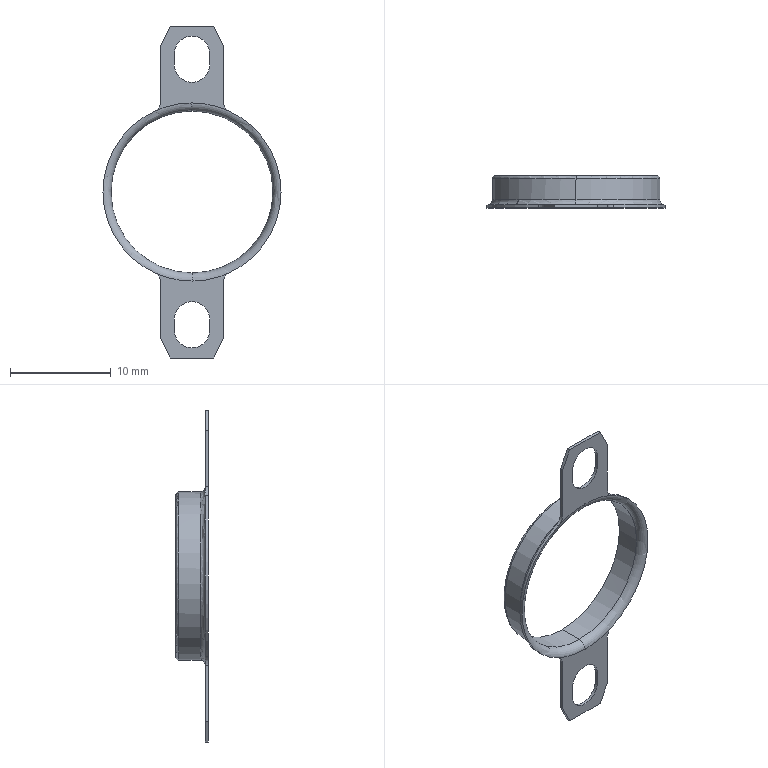Part | STEP file | WENKONGZHIJIA_3_1 | 1 solid | 38 faces | box 17.7 x 3.2 x 33 mm | volume 72.757 mm3 | plane 18 | cylinder 14 | torus 6 | commonest cylinder face diameters 2 x4 3.5 x4 16.1 x2 16.7 x2 17.7 x2
STEP:
#1=CARTESIAN_POINT('',(0.,0.,0.));
#2=DIRECTION('',(0.,0.,1.));
#3=DIRECTION('',(1.,0.,0.));
#4=AXIS2_PLACEMENT_3D('',#1,#2,#3);
#5=CARTESIAN_POINT('',(3.729,0.,8.026));
#6=VERTEX_POINT('',#5);
#7=CARTESIAN_POINT('',(0.,0.,8.85));
#8=VERTEX_POINT('',#7);
#9=CARTESIAN_POINT('',(0.,0.,0.));
#10=DIRECTION('',(0.,-1.,0.));
#11=DIRECTION('',(0.4213,0.,0.9069));
#12=AXIS2_PLACEMENT_3D('',#9,#10,#11);
#13=CIRCLE('',#12,8.85);
#14=EDGE_CURVE('',#6,#8,#13,.T.);
#15=ORIENTED_EDGE('',*,*,#14,.T.);
#16=CARTESIAN_POINT('',(-0.09026,0.,8.85));
#17=VERTEX_POINT('',#16);
#18=CARTESIAN_POINT('',(0.,0.,0.));
#19=DIRECTION('',(0.,1.,0.));
#20=DIRECTION('',(-0.0102,0.,0.9999));
#21=AXIS2_PLACEMENT_3D('',#18,#19,#20);
#22=CIRCLE('',#21,8.85);
#23=EDGE_CURVE('',#17,#8,#22,.T.);
#24=ORIENTED_EDGE('',*,*,#23,.F.);
#25=CARTESIAN_POINT('',(-3.729,0.,8.026));
#26=VERTEX_POINT('',#25);
#27=CARTESIAN_POINT('',(0.,0.,0.));
#28=DIRECTION('',(0.,-1.,0.));
#29=DIRECTION('',(-0.0102,0.,0.9999));
#30=AXIS2_PLACEMENT_3D('',#27,#28,#29);
#31=CIRCLE('',#30,8.85);
#32=EDGE_CURVE('',#17,#26,#31,.T.);
#33=ORIENTED_EDGE('',*,*,#32,.T.);
#34=CARTESIAN_POINT('',(-3.15,0.,8.933));
#35=VERTEX_POINT('',#34);
#36=CARTESIAN_POINT('',(-4.15,0.,8.933));
#37=DIRECTION('',(0.,-1.,0.));
#38=DIRECTION('',(0.4213,0.,-0.9069));
#39=AXIS2_PLACEMENT_3D('',#36,#37,#38);
#40=CIRCLE('',#39,1.);
#41=EDGE_CURVE('',#26,#35,#40,.T.);
#42=ORIENTED_EDGE('',*,*,#41,.T.);
#43=CARTESIAN_POINT('',(-3.15,0.,14.5));
#44=VERTEX_POINT('',#43);
#45=CARTESIAN_POINT('',(-3.15,0.,14.5));
#46=DIRECTION('',(0.,0.,-1.));
#47=VECTOR('',#46,5.567);
#48=LINE('',#45,#47);
#49=EDGE_CURVE('',#44,#35,#48,.T.);
#50=ORIENTED_EDGE('',*,*,#49,.F.);
#51=CARTESIAN_POINT('',(-2.15,0.,16.5));
#52=VERTEX_POINT('',#51);
#53=CARTESIAN_POINT('',(-3.15,0.,14.5));
#54=DIRECTION('',(0.4472,0.,0.8944));
#55=VECTOR('',#54,2.236);
#56=LINE('',#53,#55);
#57=EDGE_CURVE('',#44,#52,#56,.T.);
#58=ORIENTED_EDGE('',*,*,#57,.T.);
#59=CARTESIAN_POINT('',(2.15,0.,16.5));
#60=VERTEX_POINT('',#59);
#61=CARTESIAN_POINT('',(2.15,0.,16.5));
#62=DIRECTION('',(-1.,0.,0.));
#63=VECTOR('',#62,4.3);
#64=LINE('',#61,#63);
#65=EDGE_CURVE('',#60,#52,#64,.T.);
#66=ORIENTED_EDGE('',*,*,#65,.F.);
#67=CARTESIAN_POINT('',(3.15,0.,14.5));
#68=VERTEX_POINT('',#67);
#69=CARTESIAN_POINT('',(2.15,0.,16.5));
#70=DIRECTION('',(0.4472,0.,-0.8944));
#71=VECTOR('',#70,2.236);
#72=LINE('',#69,#71);
#73=EDGE_CURVE('',#60,#68,#72,.T.);
#74=ORIENTED_EDGE('',*,*,#73,.T.);
#75=CARTESIAN_POINT('',(3.15,0.,8.933));
#76=VERTEX_POINT('',#75);
#77=CARTESIAN_POINT('',(3.15,0.,8.933));
#78=DIRECTION('',(0.,0.,1.));
#79=VECTOR('',#78,5.567);
#80=LINE('',#77,#79);
#81=EDGE_CURVE('',#76,#68,#80,.T.);
#82=ORIENTED_EDGE('',*,*,#81,.F.);
#83=CARTESIAN_POINT('',(4.15,0.,8.933));
#84=DIRECTION('',(0.,-1.,0.));
#85=DIRECTION('',(-1.,0.,0.));
#86=AXIS2_PLACEMENT_3D('',#83,#84,#85);
#87=CIRCLE('',#86,1.);
#88=EDGE_CURVE('',#76,#6,#87,.T.);
#89=ORIENTED_EDGE('',*,*,#88,.T.);
#90=EDGE_LOOP('',(#15,#24,#33,#42,#50,#58,#66,#74,#82,#89));
#91=FACE_OUTER_BOUND('',#90,.F.);
#92=CARTESIAN_POINT('',(1.75,0.,13.75));
#93=VERTEX_POINT('',#92);
#94=CARTESIAN_POINT('',(0.,0.,15.5));
#95=VERTEX_POINT('',#94);
#96=CARTESIAN_POINT('',(0.,0.,13.75));
#97=DIRECTION('',(0.,-1.,0.));
#98=DIRECTION('',(1.,0.,0.));
#99=AXIS2_PLACEMENT_3D('',#96,#97,#98);
#100=CIRCLE('',#99,1.75);
#101=EDGE_CURVE('',#93,#95,#100,.T.);
#102=ORIENTED_EDGE('',*,*,#101,.T.);
#103=CARTESIAN_POINT('',(-1.75,0.,13.75));
#104=VERTEX_POINT('',#103);
#105=CARTESIAN_POINT('',(0.,0.,13.75));
#106=DIRECTION('',(0.,-1.,0.));
#107=DIRECTION('',(0.,0.,1.));
#108=AXIS2_PLACEMENT_3D('',#105,#106,#107);
#109=CIRCLE('',#108,1.75);
#110=EDGE_CURVE('',#95,#104,#109,.T.);
#111=ORIENTED_EDGE('',*,*,#110,.T.);
#112=CARTESIAN_POINT('',(-1.75,0.,12.65));
#113=VERTEX_POINT('',#112);
#114=CARTESIAN_POINT('',(-1.75,0.,12.65));
#115=DIRECTION('',(0.,0.,1.));
#116=VECTOR('',#115,1.1);
#117=LINE('',#114,#116);
#118=EDGE_CURVE('',#113,#104,#117,.T.);
#119=ORIENTED_EDGE('',*,*,#118,.F.);
#120=CARTESIAN_POINT('',(0.,0.,10.9));
#121=VERTEX_POINT('',#120);
#122=CARTESIAN_POINT('',(0.,0.,12.65));
#123=DIRECTION('',(0.,-1.,0.));
#124=DIRECTION('',(-1.,0.,0.));
#125=AXIS2_PLACEMENT_3D('',#122,#123,#124);
#126=CIRCLE('',#125,1.75);
#127=EDGE_CURVE('',#113,#121,#126,.T.);
#128=ORIENTED_EDGE('',*,*,#127,.T.);
#129=CARTESIAN_POINT('',(1.75,0.,12.65));
#130=VERTEX_POINT('',#129);
#131=CARTESIAN_POINT('',(0.,0.,12.65));
#132=DIRECTION('',(0.,-1.,0.));
#133=DIRECTION('',(0.,0.,-1.));
#134=AXIS2_PLACEMENT_3D('',#131,#132,#133);
#135=CIRCLE('',#134,1.75);
#136=EDGE_CURVE('',#121,#130,#135,.T.);
#137=ORIENTED_EDGE('',*,*,#136,.T.);
#138=CARTESIAN_POINT('',(1.75,0.,13.75));
#139=DIRECTION('',(0.,0.,-1.));
#140=VECTOR('',#139,1.1);
#141=LINE('',#138,#140);
#142=EDGE_CURVE('',#93,#130,#141,.T.);
#143=ORIENTED_EDGE('',*,*,#142,.F.);
#144=EDGE_LOOP('',(#102,#111,#119,#128,#137,#143));
#145=FACE_BOUND('',#144,.F.);
#146=CARTESIAN_POINT('',(0.,0.,0.));
#147=DIRECTION('',(0.,1.,0.));
#148=DIRECTION('',(1.,0.,0.));
#149=AXIS2_PLACEMENT_3D('',#146,#147,#148);
#150=PLANE('',#149);
#151=ADVANCED_FACE('',(#91,#145),#150,.F.);
#152=ORIENTED_EDGE('',*,*,#14,.F.);
#153=CARTESIAN_POINT('',(8.85,0.,0.));
#154=VERTEX_POINT('',#153);
#155=CARTESIAN_POINT('',(0.,0.,0.));
#156=DIRECTION('',(0.,1.,0.));
#157=DIRECTION('',(0.4213,0.,0.9069));
#158=AXIS2_PLACEMENT_3D('',#155,#156,#157);
#159=CIRCLE('',#158,8.85);
#160=EDGE_CURVE('',#6,#154,#159,.T.);
#161=ORIENTED_EDGE('',*,*,#160,.T.);
#162=CARTESIAN_POINT('',(3.729,0.,-8.026));
#163=VERTEX_POINT('',#162);
#164=CARTESIAN_POINT('',(0.,0.,0.));
#165=DIRECTION('',(0.,1.,0.));
#166=DIRECTION('',(1.,0.,0.));
#167=AXIS2_PLACEMENT_3D('',#164,#165,#166);
#168=CIRCLE('',#167,8.85);
#169=EDGE_CURVE('',#154,#163,#168,.T.);
#170=ORIENTED_EDGE('',*,*,#169,.T.);
#171=CARTESIAN_POINT('',(0.09026,0.,-8.85));
#172=VERTEX_POINT('',#171);
#173=CARTESIAN_POINT('',(0.,0.,0.));
#174=DIRECTION('',(0.,-1.,0.));
#175=DIRECTION('',(0.0102,0.,-0.9999));
#176=AXIS2_PLACEMENT_3D('',#173,#174,#175);
#177=CIRCLE('',#176,8.85);
#178=EDGE_CURVE('',#172,#163,#177,.T.);
#179=ORIENTED_EDGE('',*,*,#178,.F.);
#180=CARTESIAN_POINT('',(0.,0.,-8.85));
#181=VERTEX_POINT('',#180);
#182=CARTESIAN_POINT('',(0.,0.,0.));
#183=DIRECTION('',(0.,1.,0.));
#184=DIRECTION('',(0.0102,0.,-0.9999));
#185=AXIS2_PLACEMENT_3D('',#182,#183,#184);
#186=CIRCLE('',#185,8.85);
#187=EDGE_CURVE('',#172,#181,#186,.T.);
#188=ORIENTED_EDGE('',*,*,#187,.T.);
#189=CARTESIAN_POINT('',(0.,0.8,-8.05));
#190=VERTEX_POINT('',#189);
#191=CARTESIAN_POINT('',(0.,0.8,-8.85));
#192=DIRECTION('',(-1.,0.,0.));
#193=DIRECTION('',(0.,-1.,0.));
#194=AXIS2_PLACEMENT_3D('',#191,#192,#193);
#195=CIRCLE('',#194,0.8);
#196=EDGE_CURVE('',#181,#190,#195,.T.);
#197=ORIENTED_EDGE('',*,*,#196,.T.);
#198=CARTESIAN_POINT('',(0.08211,0.8,-8.05));
#199=VERTEX_POINT('',#198);
#200=CARTESIAN_POINT('',(0.,0.8,0.));
#201=DIRECTION('',(0.,-1.,0.));
#202=DIRECTION('',(0.,0.,-1.));
#203=AXIS2_PLACEMENT_3D('',#200,#201,#202);
#204=CIRCLE('',#203,8.05);
#205=EDGE_CURVE('',#190,#199,#204,.T.);
#206=ORIENTED_EDGE('',*,*,#205,.T.);
#207=CARTESIAN_POINT('',(0.,0.8,8.05));
#208=VERTEX_POINT('',#207);
#209=CARTESIAN_POINT('',(0.,0.8,0.));
#210=DIRECTION('',(0.,-1.,0.));
#211=DIRECTION('',(0.0102,0.,-0.9999));
#212=AXIS2_PLACEMENT_3D('',#209,#210,#211);
#213=CIRCLE('',#212,8.05);
#214=EDGE_CURVE('',#199,#208,#213,.T.);
#215=ORIENTED_EDGE('',*,*,#214,.T.);
#216=CARTESIAN_POINT('',(0.,0.8,8.85));
#217=DIRECTION('',(1.,0.,0.));
#218=DIRECTION('',(0.,-1.,0.));
#219=AXIS2_PLACEMENT_3D('',#216,#217,#218);
#220=CIRCLE('',#219,0.8);
#221=EDGE_CURVE('',#8,#208,#220,.T.);
#222=ORIENTED_EDGE('',*,*,#221,.F.);
#223=EDGE_LOOP('',(#152,#161,#170,#179,#188,#197,#206,#215,#222));
#224=FACE_OUTER_BOUND('',#223,.F.);
#225=CARTESIAN_POINT('',(0.,0.8,0.));
#226=DIRECTION('',(0.,-1.,0.));
#227=DIRECTION('',(-0.0102,0.,0.9999));
#228=AXIS2_PLACEMENT_3D('',#225,#226,#227);
#229=TOROIDAL_SURFACE('',#228,8.85,0.8);
#230=ADVANCED_FACE('',(#224),#229,.T.);
#231=CARTESIAN_POINT('',(8.85,0.3,0.));
#232=VERTEX_POINT('',#231);
#233=CARTESIAN_POINT('',(3.729,0.3,8.026));
#234=VERTEX_POINT('',#233);
#235=CARTESIAN_POINT('',(0.,0.3,0.));
#236=DIRECTION('',(0.,-1.,0.));
#237=DIRECTION('',(1.,0.,0.));
#238=AXIS2_PLACEMENT_3D('',#235,#236,#237);
#239=CIRCLE('',#238,8.85);
#240=EDGE_CURVE('',#232,#234,#239,.T.);
#241=ORIENTED_EDGE('',*,*,#240,.F.);
#242=CARTESIAN_POINT('',(3.729,0.3,-8.026));
#243=VERTEX_POINT('',#242);
#244=CARTESIAN_POINT('',(0.,0.3,0.));
#245=DIRECTION('',(0.,-1.,0.));
#246=DIRECTION('',(0.4213,0.,-0.9069));
#247=AXIS2_PLACEMENT_3D('',#244,#245,#246);
#248=CIRCLE('',#247,8.85);
#249=EDGE_CURVE('',#243,#232,#248,.T.);
#250=ORIENTED_EDGE('',*,*,#249,.F.);
#251=CARTESIAN_POINT('',(3.729,0.3,-8.026));
#252=DIRECTION('',(0.,-1.,0.));
#253=VECTOR('',#252,0.3);
#254=LINE('',#251,#253);
#255=EDGE_CURVE('',#243,#163,#254,.T.);
#256=ORIENTED_EDGE('',*,*,#255,.T.);
#257=ORIENTED_EDGE('',*,*,#169,.F.);
#258=ORIENTED_EDGE('',*,*,#160,.F.);
#259=CARTESIAN_POINT('',(3.729,0.,8.026));
#260=DIRECTION('',(0.,1.,0.));
#261=VECTOR('',#260,0.3);
#262=LINE('',#259,#261);
#263=EDGE_CURVE('',#6,#234,#262,.T.);
#264=ORIENTED_EDGE('',*,*,#263,.T.);
#265=EDGE_LOOP('',(#241,#250,#256,#257,#258,#264));
#266=FACE_OUTER_BOUND('',#265,.F.);
#267=CARTESIAN_POINT('',(0.,0.,0.));
#268=DIRECTION('',(0.,1.,0.));
#269=DIRECTION('',(1.,0.,0.));
#270=AXIS2_PLACEMENT_3D('',#267,#268,#269);
#271=CYLINDRICAL_SURFACE('',#270,8.85);
#272=ADVANCED_FACE('',(#266),#271,.T.);
#273=CARTESIAN_POINT('',(0.,0.3,-8.85));
#274=VERTEX_POINT('',#273);
#275=CARTESIAN_POINT('',(0.06126,0.3,-8.85));
#276=VERTEX_POINT('',#275);
#277=CARTESIAN_POINT('',(0.,0.3,0.));
#278=DIRECTION('',(0.,-1.,0.));
#279=DIRECTION('',(0.,0.,-1.));
#280=AXIS2_PLACEMENT_3D('',#277,#278,#279);
#281=CIRCLE('',#280,8.85);
#282=EDGE_CURVE('',#274,#276,#281,.T.);
#283=ORIENTED_EDGE('',*,*,#282,.T.);
#284=CARTESIAN_POINT('',(0.,0.3,0.));
#285=DIRECTION('',(0.,1.,0.));
#286=DIRECTION('',(0.4213,0.,-0.9069));
#287=AXIS2_PLACEMENT_3D('',#284,#285,#286);
#288=CIRCLE('',#287,8.85);
#289=EDGE_CURVE('',#243,#276,#288,.T.);
#290=ORIENTED_EDGE('',*,*,#289,.F.);
#291=ORIENTED_EDGE('',*,*,#249,.T.);
#292=ORIENTED_EDGE('',*,*,#240,.T.);
#293=CARTESIAN_POINT('',(0.,0.3,8.85));
#294=VERTEX_POINT('',#293);
#295=CARTESIAN_POINT('',(0.,0.3,0.));
#296=DIRECTION('',(0.,1.,0.));
#297=DIRECTION('',(0.,0.,1.));
#298=AXIS2_PLACEMENT_3D('',#295,#296,#297);
#299=CIRCLE('',#298,8.85);
#300=EDGE_CURVE('',#294,#234,#299,.T.);
#301=ORIENTED_EDGE('',*,*,#300,.F.);
#302=CARTESIAN_POINT('',(0.,0.8,8.35));
#303=VERTEX_POINT('',#302);
#304=CARTESIAN_POINT('',(0.,0.8,8.85));
#305=DIRECTION('',(1.,0.,0.));
#306=DIRECTION('',(0.,-1.,0.));
#307=AXIS2_PLACEMENT_3D('',#304,#305,#306);
#308=CIRCLE('',#307,0.5);
#309=EDGE_CURVE('',#294,#303,#308,.T.);
#310=ORIENTED_EDGE('',*,*,#309,.T.);
#311=CARTESIAN_POINT('',(0.0578,0.8,-8.35));
#312=VERTEX_POINT('',#311);
#313=CARTESIAN_POINT('',(0.,0.8,0.));
#314=DIRECTION('',(0.,1.,0.));
#315=DIRECTION('',(0.,0.,1.));
#316=AXIS2_PLACEMENT_3D('',#313,#314,#315);
#317=CIRCLE('',#316,8.35);
#318=EDGE_CURVE('',#303,#312,#317,.T.);
#319=ORIENTED_EDGE('',*,*,#318,.T.);
#320=CARTESIAN_POINT('',(0.,0.8,-8.35));
#321=VERTEX_POINT('',#320);
#322=CARTESIAN_POINT('',(0.,0.8,0.));
#323=DIRECTION('',(0.,1.,0.));
#324=DIRECTION('',(0.006922,0.,-1.));
#325=AXIS2_PLACEMENT_3D('',#322,#323,#324);
#326=CIRCLE('',#325,8.35);
#327=EDGE_CURVE('',#312,#321,#326,.T.);
#328=ORIENTED_EDGE('',*,*,#327,.T.);
#329=CARTESIAN_POINT('',(0.,0.8,-8.85));
#330=DIRECTION('',(-1.,0.,0.));
#331=DIRECTION('',(0.,-1.,0.));
#332=AXIS2_PLACEMENT_3D('',#329,#330,#331);
#333=CIRCLE('',#332,0.5);
#334=EDGE_CURVE('',#274,#321,#333,.T.);
#335=ORIENTED_EDGE('',*,*,#334,.F.);
#336=EDGE_LOOP('',(#283,#290,#291,#292,#301,#310,#319,#328,#335));
#337=FACE_OUTER_BOUND('',#336,.F.);
#338=CARTESIAN_POINT('',(0.,0.8,0.));
#339=DIRECTION('',(0.,1.,0.));
#340=DIRECTION('',(-0.006922,0.,1.));
#341=AXIS2_PLACEMENT_3D('',#338,#339,#340);
#342=TOROIDAL_SURFACE('',#341,8.85,0.5);
#343=ADVANCED_FACE('',(#337),#342,.F.);
#344=ORIENTED_EDGE('',*,*,#289,.T.);
#345=ORIENTED_EDGE('',*,*,#282,.F.);
#346=CARTESIAN_POINT('',(-3.729,0.3,-8.026));
#347=VERTEX_POINT('',#346);
#348=CARTESIAN_POINT('',(0.,0.3,0.));
#349=DIRECTION('',(0.,1.,0.));
#350=DIRECTION('',(0.,0.,-1.));
#351=AXIS2_PLACEMENT_3D('',#348,#349,#350);
#352=CIRCLE('',#351,8.85);
#353=EDGE_CURVE('',#274,#347,#352,.T.);
#354=ORIENTED_EDGE('',*,*,#353,.T.);
#355=CARTESIAN_POINT('',(-3.15,0.3,-8.933));
#356=VERTEX_POINT('',#355);
#357=CARTESIAN_POINT('',(-4.15,0.3,-8.933));
#358=DIRECTION('',(0.,1.,0.));
#359=DIRECTION('',(0.4213,0.,0.9069));
#360=AXIS2_PLACEMENT_3D('',#357,#358,#359);
#361=CIRCLE('',#360,1.);
#362=EDGE_CURVE('',#347,#356,#361,.T.);
#363=ORIENTED_EDGE('',*,*,#362,.T.);
#364=CARTESIAN_POINT('',(-3.15,0.3,-14.5));
#365=VERTEX_POINT('',#364);
#366=CARTESIAN_POINT('',(-3.15,0.3,-8.933));
#367=DIRECTION('',(0.,0.,-1.));
#368=VECTOR('',#367,5.567);
#369=LINE('',#366,#368);
#370=EDGE_CURVE('',#356,#365,#369,.T.);
#371=ORIENTED_EDGE('',*,*,#370,.T.);
#372=CARTESIAN_POINT('',(-2.15,0.3,-16.5));
#373=VERTEX_POINT('',#372);
#374=CARTESIAN_POINT('',(-3.15,0.3,-14.5));
#375=DIRECTION('',(0.4472,0.,-0.8944));
#376=VECTOR('',#375,2.236);
#377=LINE('',#374,#376);
#378=EDGE_CURVE('',#365,#373,#377,.T.);
#379=ORIENTED_EDGE('',*,*,#378,.T.);
#380=CARTESIAN_POINT('',(2.15,0.3,-16.5));
#381=VERTEX_POINT('',#380);
#382=CARTESIAN_POINT('',(-2.15,0.3,-16.5));
#383=DIRECTION('',(1.,0.,0.));
#384=VECTOR('',#383,4.3);
#385=LINE('',#382,#384);
#386=EDGE_CURVE('',#373,#381,#385,.T.);
#387=ORIENTED_EDGE('',*,*,#386,.T.);
#388=CARTESIAN_POINT('',(3.15,0.3,-14.5));
#389=VERTEX_POINT('',#388);
#390=CARTESIAN_POINT('',(2.15,0.3,-16.5));
#391=DIRECTION('',(0.4472,0.,0.8944));
#392=VECTOR('',#391,2.236);
#393=LINE('',#390,#392);
#394=EDGE_CURVE('',#381,#389,#393,.T.);
#395=ORIENTED_EDGE('',*,*,#394,.T.);
#396=CARTESIAN_POINT('',(3.15,0.3,-8.933));
#397=VERTEX_POINT('',#396);
#398=CARTESIAN_POINT('',(3.15,0.3,-14.5));
#399=DIRECTION('',(0.,0.,1.));
#400=VECTOR('',#399,5.567);
#401=LINE('',#398,#400);
#402=EDGE_CURVE('',#389,#397,#401,.T.);
#403=ORIENTED_EDGE('',*,*,#402,.T.);
#404=CARTESIAN_POINT('',(4.15,0.3,-8.933));
#405=DIRECTION('',(0.,1.,0.));
#406=DIRECTION('',(-1.,0.,0.));
#407=AXIS2_PLACEMENT_3D('',#404,#405,#406);
#408=CIRCLE('',#407,1.);
#409=EDGE_CURVE('',#397,#243,#408,.T.);
#410=ORIENTED_EDGE('',*,*,#409,.T.);
#411=EDGE_LOOP('',(#344,#345,#354,#363,#371,#379,#387,#395,#403,#410));
#412=FACE_OUTER_BOUND('',#411,.F.);
#413=CARTESIAN_POINT('',(-1.75,0.3,-12.65));
#414=VERTEX_POINT('',#413);
#415=CARTESIAN_POINT('',(0.,0.3,-10.9));
#416=VERTEX_POINT('',#415);
#417=CARTESIAN_POINT('',(0.,0.3,-12.65));
#418=DIRECTION('',(0.,1.,0.));
#419=DIRECTION('',(-1.,0.,0.));
#420=AXIS2_PLACEMENT_3D('',#417,#418,#419);
#421=CIRCLE('',#420,1.75);
#422=EDGE_CURVE('',#414,#416,#421,.T.);
#423=ORIENTED_EDGE('',*,*,#422,.T.);
#424=CARTESIAN_POINT('',(1.75,0.3,-12.65));
#425=VERTEX_POINT('',#424);
#426=CARTESIAN_POINT('',(0.,0.3,-12.65));
#427=DIRECTION('',(0.,1.,0.));
#428=DIRECTION('',(0.,0.,1.));
#429=AXIS2_PLACEMENT_3D('',#426,#427,#428);
#430=CIRCLE('',#429,1.75);
#431=EDGE_CURVE('',#416,#425,#430,.T.);
#432=ORIENTED_EDGE('',*,*,#431,.T.);
#433=CARTESIAN_POINT('',(1.75,0.3,-13.75));
#434=VERTEX_POINT('',#433);
#435=CARTESIAN_POINT('',(1.75,0.3,-12.65));
#436=DIRECTION('',(0.,0.,-1.));
#437=VECTOR('',#436,1.1);
#438=LINE('',#435,#437);
#439=EDGE_CURVE('',#425,#434,#438,.T.);
#440=ORIENTED_EDGE('',*,*,#439,.T.);
#441=CARTESIAN_POINT('',(0.,0.3,-15.5));
#442=VERTEX_POINT('',#441);
#443=CARTESIAN_POINT('',(0.,0.3,-13.75));
#444=DIRECTION('',(0.,1.,0.));
#445=DIRECTION('',(1.,0.,0.));
#446=AXIS2_PLACEMENT_3D('',#443,#444,#445);
#447=CIRCLE('',#446,1.75);
#448=EDGE_CURVE('',#434,#442,#447,.T.);
#449=ORIENTED_EDGE('',*,*,#448,.T.);
#450=CARTESIAN_POINT('',(-1.75,0.3,-13.75));
#451=VERTEX_POINT('',#450);
#452=CARTESIAN_POINT('',(0.,0.3,-13.75));
#453=DIRECTION('',(0.,1.,0.));
#454=DIRECTION('',(0.,0.,-1.));
#455=AXIS2_PLACEMENT_3D('',#452,#453,#454);
#456=CIRCLE('',#455,1.75);
#457=EDGE_CURVE('',#442,#451,#456,.T.);
#458=ORIENTED_EDGE('',*,*,#457,.T.);
#459=CARTESIAN_POINT('',(-1.75,0.3,-13.75));
#460=DIRECTION('',(0.,0.,1.));
#461=VECTOR('',#460,1.1);
#462=LINE('',#459,#461);
#463=EDGE_CURVE('',#451,#414,#462,.T.);
#464=ORIENTED_EDGE('',*,*,#463,.T.);
#465=EDGE_LOOP('',(#423,#432,#440,#449,#458,#464));
#466=FACE_BOUND('',#465,.F.);
#467=CARTESIAN_POINT('',(0.,0.3,0.));
#468=DIRECTION('',(0.,-1.,0.));
#469=DIRECTION('',(0.,0.,1.));
#470=AXIS2_PLACEMENT_3D('',#467,#468,#469);
#471=PLANE('',#470);
#472=ADVANCED_FACE('',(#412,#466),#471,.F.);
#473=CARTESIAN_POINT('',(-0.06126,0.3,8.85));
#474=VERTEX_POINT('',#473);
#475=CARTESIAN_POINT('',(0.,0.3,0.));
#476=DIRECTION('',(0.,-1.,0.));
#477=DIRECTION('',(0.,0.,1.));
#478=AXIS2_PLACEMENT_3D('',#475,#476,#477);
#479=CIRCLE('',#478,8.85);
#480=EDGE_CURVE('',#294,#474,#479,.T.);
#481=ORIENTED_EDGE('',*,*,#480,.T.);
#482=CARTESIAN_POINT('',(-3.729,0.3,8.026));
#483=VERTEX_POINT('',#482);
#484=CARTESIAN_POINT('',(0.,0.3,0.));
#485=DIRECTION('',(0.,1.,0.));
#486=DIRECTION('',(-0.4213,0.,0.9069));
#487=AXIS2_PLACEMENT_3D('',#484,#485,#486);
#488=CIRCLE('',#487,8.85);
#489=EDGE_CURVE('',#483,#474,#488,.T.);
#490=ORIENTED_EDGE('',*,*,#489,.F.);
#491=CARTESIAN_POINT('',(-8.85,0.3,0.));
#492=VERTEX_POINT('',#491);
#493=CARTESIAN_POINT('',(0.,0.3,0.));
#494=DIRECTION('',(0.,-1.,0.));
#495=DIRECTION('',(-0.4213,0.,0.9069));
#496=AXIS2_PLACEMENT_3D('',#493,#494,#495);
#497=CIRCLE('',#496,8.85);
#498=EDGE_CURVE('',#483,#492,#497,.T.);
#499=ORIENTED_EDGE('',*,*,#498,.T.);
#500=CARTESIAN_POINT('',(0.,0.3,0.));
#501=DIRECTION('',(0.,-1.,0.));
#502=DIRECTION('',(-1.,0.,0.));
#503=AXIS2_PLACEMENT_3D('',#500,#501,#502);
#504=CIRCLE('',#503,8.85);
#505=EDGE_CURVE('',#492,#347,#504,.T.);
#506=ORIENTED_EDGE('',*,*,#505,.T.);
#507=ORIENTED_EDGE('',*,*,#353,.F.);
#508=ORIENTED_EDGE('',*,*,#334,.T.);
#509=CARTESIAN_POINT('',(-0.0578,0.8,8.35));
#510=VERTEX_POINT('',#509);
#511=CARTESIAN_POINT('',(0.,0.8,0.));
#512=DIRECTION('',(0.,1.,0.));
#513=DIRECTION('',(0.,0.,-1.));
#514=AXIS2_PLACEMENT_3D('',#511,#512,#513);
#515=CIRCLE('',#514,8.35);
#516=EDGE_CURVE('',#321,#510,#515,.T.);
#517=ORIENTED_EDGE('',*,*,#516,.T.);
#518=CARTESIAN_POINT('',(0.,0.8,0.));
#519=DIRECTION('',(0.,1.,0.));
#520=DIRECTION('',(-0.006922,0.,1.));
#521=AXIS2_PLACEMENT_3D('',#518,#519,#520);
#522=CIRCLE('',#521,8.35);
#523=EDGE_CURVE('',#510,#303,#522,.T.);
#524=ORIENTED_EDGE('',*,*,#523,.T.);
#525=ORIENTED_EDGE('',*,*,#309,.F.);
#526=EDGE_LOOP('',(#481,#490,#499,#506,#507,#508,#517,#524,#525));
#527=FACE_OUTER_BOUND('',#526,.F.);
#528=CARTESIAN_POINT('',(0.,0.8,0.));
#529=DIRECTION('',(0.,1.,0.));
#530=DIRECTION('',(0.006922,0.,-1.));
#531=AXIS2_PLACEMENT_3D('',#528,#529,#530);
#532=TOROIDAL_SURFACE('',#531,8.85,0.5);
#533=ADVANCED_FACE('',(#527),#532,.F.);
#534=ORIENTED_EDGE('',*,*,#300,.T.);
#535=CARTESIAN_POINT('',(3.15,0.3,8.933));
#536=VERTEX_POINT('',#535);
#537=CARTESIAN_POINT('',(4.15,0.3,8.933));
#538=DIRECTION('',(0.,1.,0.));
#539=DIRECTION('',(-0.4213,0.,-0.9069));
#540=AXIS2_PLACEMENT_3D('',#537,#538,#539);
#541=CIRCLE('',#540,1.);
#542=EDGE_CURVE('',#234,#536,#541,.T.);
#543=ORIENTED_EDGE('',*,*,#542,.T.);
#544=CARTESIAN_POINT('',(3.15,0.3,14.5));
#545=VERTEX_POINT('',#544);
#546=CARTESIAN_POINT('',(3.15,0.3,14.5));
#547=DIRECTION('',(0.,0.,-1.));
#548=VECTOR('',#547,5.567);
#549=LINE('',#546,#548);
#550=EDGE_CURVE('',#545,#536,#549,.T.);
#551=ORIENTED_EDGE('',*,*,#550,.F.);
#552=CARTESIAN_POINT('',(2.15,0.3,16.5));
#553=VERTEX_POINT('',#552);
#554=CARTESIAN_POINT('',(3.15,0.3,14.5));
#555=DIRECTION('',(-0.4472,0.,0.8944));
#556=VECTOR('',#555,2.236);
#557=LINE('',#554,#556);
#558=EDGE_CURVE('',#545,#553,#557,.T.);
#559=ORIENTED_EDGE('',*,*,#558,.T.);
#560=CARTESIAN_POINT('',(-2.15,0.3,16.5));
#561=VERTEX_POINT('',#560);
#562=CARTESIAN_POINT('',(2.15,0.3,16.5));
#563=DIRECTION('',(-1.,0.,0.));
#564=VECTOR('',#563,4.3);
#565=LINE('',#562,#564);
#566=EDGE_CURVE('',#553,#561,#565,.T.);
#567=ORIENTED_EDGE('',*,*,#566,.T.);
#568=CARTESIAN_POINT('',(-3.15,0.3,14.5));
#569=VERTEX_POINT('',#568);
#570=CARTESIAN_POINT('',(-2.15,0.3,16.5));
#571=DIRECTION('',(-0.4472,0.,-0.8944));
#572=VECTOR('',#571,2.236);
#573=LINE('',#570,#572);
#574=EDGE_CURVE('',#561,#569,#573,.T.);
#575=ORIENTED_EDGE('',*,*,#574,.T.);
#576=CARTESIAN_POINT('',(-3.15,0.3,8.933));
#577=VERTEX_POINT('',#576);
#578=CARTESIAN_POINT('',(-3.15,0.3,14.5));
#579=DIRECTION('',(0.,0.,-1.));
#580=VECTOR('',#579,5.567);
#581=LINE('',#578,#580);
#582=EDGE_CURVE('',#569,#577,#581,.T.);
#583=ORIENTED_EDGE('',*,*,#582,.T.);
#584=CARTESIAN_POINT('',(-4.15,0.3,8.933));
#585=DIRECTION('',(0.,1.,0.));
#586=DIRECTION('',(1.,0.,0.));
#587=AXIS2_PLACEMENT_3D('',#584,#585,#586);
#588=CIRCLE('',#587,1.);
#589=EDGE_CURVE('',#577,#483,#588,.T.);
#590=ORIENTED_EDGE('',*,*,#589,.T.);
#591=ORIENTED_EDGE('',*,*,#489,.T.);
#592=ORIENTED_EDGE('',*,*,#480,.F.);
#593=EDGE_LOOP('',(#534,#543,#551,#559,#567,#575,#583,#590,#591,#592));
#594=FACE_OUTER_BOUND('',#593,.F.);
#595=CARTESIAN_POINT('',(-1.75,0.3,13.75));
#596=VERTEX_POINT('',#595);
#597=CARTESIAN_POINT('',(0.,0.3,15.5));
#598=VERTEX_POINT('',#597);
#599=CARTESIAN_POINT('',(0.,0.3,13.75));
#600=DIRECTION('',(0.,1.,0.));
#601=DIRECTION('',(-1.,0.,0.));
#602=AXIS2_PLACEMENT_3D('',#599,#600,#601);
#603=CIRCLE('',#602,1.75);
#604=EDGE_CURVE('',#596,#598,#603,.T.);
#605=ORIENTED_EDGE('',*,*,#604,.T.);
#606=CARTESIAN_POINT('',(1.75,0.3,13.75));
#607=VERTEX_POINT('',#606);
#608=CARTESIAN_POINT('',(0.,0.3,13.75));
#609=DIRECTION('',(0.,1.,0.));
#610=DIRECTION('',(0.,0.,1.));
#611=AXIS2_PLACEMENT_3D('',#608,#609,#610);
#612=CIRCLE('',#611,1.75);
#613=EDGE_CURVE('',#598,#607,#612,.T.);
#614=ORIENTED_EDGE('',*,*,#613,.T.);
#615=CARTESIAN_POINT('',(1.75,0.3,12.65));
#616=VERTEX_POINT('',#615);
#617=CARTESIAN_POINT('',(1.75,0.3,13.75));
#618=DIRECTION('',(0.,0.,-1.));
#619=VECTOR('',#618,1.1);
#620=LINE('',#617,#619);
#621=EDGE_CURVE('',#607,#616,#620,.T.);
#622=ORIENTED_EDGE('',*,*,#621,.T.);
#623=CARTESIAN_POINT('',(0.,0.3,10.9));
#624=VERTEX_POINT('',#623);
#625=CARTESIAN_POINT('',(0.,0.3,12.65));
#626=DIRECTION('',(0.,1.,0.));
#627=DIRECTION('',(1.,0.,0.));
#628=AXIS2_PLACEMENT_3D('',#625,#626,#627);
#629=CIRCLE('',#628,1.75);
#630=EDGE_CURVE('',#616,#624,#629,.T.);
#631=ORIENTED_EDGE('',*,*,#630,.T.);
#632=CARTESIAN_POINT('',(-1.75,0.3,12.65));
#633=VERTEX_POINT('',#632);
#634=CARTESIAN_POINT('',(0.,0.3,12.65));
#635=DIRECTION('',(0.,1.,0.));
#636=DIRECTION('',(0.,0.,-1.));
#637=AXIS2_PLACEMENT_3D('',#634,#635,#636);
#638=CIRCLE('',#637,1.75);
#639=EDGE_CURVE('',#624,#633,#638,.T.);
#640=ORIENTED_EDGE('',*,*,#639,.T.);
#641=CARTESIAN_POINT('',(-1.75,0.3,12.65));
#642=DIRECTION('',(0.,0.,1.));
#643=VECTOR('',#642,1.1);
#644=LINE('',#641,#643);
#645=EDGE_CURVE('',#633,#596,#644,.T.);
#646=ORIENTED_EDGE('',*,*,#645,.T.);
#647=EDGE_LOOP('',(#605,#614,#622,#631,#640,#646));
#648=FACE_BOUND('',#647,.F.);
#649=CARTESIAN_POINT('',(0.,0.3,0.));
#650=DIRECTION('',(0.,-1.,0.));
#651=DIRECTION('',(0.,0.,1.));
#652=AXIS2_PLACEMENT_3D('',#649,#650,#651);
#653=PLANE('',#652);
#654=ADVANCED_FACE('',(#594,#648),#653,.F.);
#655=ORIENTED_EDGE('',*,*,#542,.F.);
#656=ORIENTED_EDGE('',*,*,#263,.F.);
#657=ORIENTED_EDGE('',*,*,#88,.F.);
#658=CARTESIAN_POINT('',(3.15,0.,8.933));
#659=DIRECTION('',(0.,1.,0.));
#660=VECTOR('',#659,0.3);
#661=LINE('',#658,#660);
#662=EDGE_CURVE('',#76,#536,#661,.T.);
#663=ORIENTED_EDGE('',*,*,#662,.T.);
#664=EDGE_LOOP('',(#655,#656,#657,#663));
#665=FACE_OUTER_BOUND('',#664,.F.);
#666=CARTESIAN_POINT('',(4.15,-4.172,8.933));
#667=DIRECTION('',(0.,1.,0.));
#668=DIRECTION('',(-0.4213,0.,-0.9069));
#669=AXIS2_PLACEMENT_3D('',#666,#667,#668);
#670=CYLINDRICAL_SURFACE('',#669,1.);
#671=ADVANCED_FACE('',(#665),#670,.F.);
#672=ORIENTED_EDGE('',*,*,#662,.F.);
#673=ORIENTED_EDGE('',*,*,#81,.T.);
#674=CARTESIAN_POINT('',(3.15,0.,14.5));
#675=DIRECTION('',(0.,1.,0.));
#676=VECTOR('',#675,0.3);
#677=LINE('',#674,#676);
#678=EDGE_CURVE('',#68,#545,#677,.T.);
#679=ORIENTED_EDGE('',*,*,#678,.T.);
#680=ORIENTED_EDGE('',*,*,#550,.T.);
#681=EDGE_LOOP('',(#672,#673,#679,#680));
#682=FACE_OUTER_BOUND('',#681,.F.);
#683=CARTESIAN_POINT('',(3.15,0.,-16.5));
#684=DIRECTION('',(1.,0.,0.));
#685=DIRECTION('',(0.,0.,1.));
#686=AXIS2_PLACEMENT_3D('',#683,#684,#685);
#687=PLANE('',#686);
#688=ADVANCED_FACE('',(#682),#687,.T.);
#689=ORIENTED_EDGE('',*,*,#558,.F.);
#690=ORIENTED_EDGE('',*,*,#678,.F.);
#691=ORIENTED_EDGE('',*,*,#73,.F.);
#692=CARTESIAN_POINT('',(2.15,0.,16.5));
#693=DIRECTION('',(0.,1.,0.));
#694=VECTOR('',#693,0.3);
#695=LINE('',#692,#694);
#696=EDGE_CURVE('',#60,#553,#695,.T.);
#697=ORIENTED_EDGE('',*,*,#696,.T.);
#698=EDGE_LOOP('',(#689,#690,#691,#697));
#699=FACE_OUTER_BOUND('',#698,.F.);
#700=CARTESIAN_POINT('',(2.65,0.15,15.5));
#701=DIRECTION('',(0.8944,0.,0.4472));
#702=DIRECTION('',(0.4472,0.,-0.8944));
#703=AXIS2_PLACEMENT_3D('',#700,#701,#702);
#704=PLANE('',#703);
#705=ADVANCED_FACE('',(#699),#704,.T.);
#706=CARTESIAN_POINT('',(-2.15,0.,16.5));
#707=DIRECTION('',(0.,1.,0.));
#708=VECTOR('',#707,0.3);
#709=LINE('',#706,#708);
#710=EDGE_CURVE('',#52,#561,#709,.T.);
#711=ORIENTED_EDGE('',*,*,#710,.T.);
#712=ORIENTED_EDGE('',*,*,#566,.F.);
#713=ORIENTED_EDGE('',*,*,#696,.F.);
#714=ORIENTED_EDGE('',*,*,#65,.T.);
#715=EDGE_LOOP('',(#711,#712,#713,#714));
#716=FACE_OUTER_BOUND('',#715,.F.);
#717=CARTESIAN_POINT('',(3.15,0.,16.5));
#718=DIRECTION('',(0.,0.,1.));
#719=DIRECTION('',(-1.,0.,0.));
#720=AXIS2_PLACEMENT_3D('',#717,#718,#719);
#721=PLANE('',#720);
#722=ADVANCED_FACE('',(#716),#721,.T.);
#723=ORIENTED_EDGE('',*,*,#574,.F.);
#724=ORIENTED_EDGE('',*,*,#710,.F.);
#725=ORIENTED_EDGE('',*,*,#57,.F.);
#726=CARTESIAN_POINT('',(-3.15,0.,14.5));
#727=DIRECTION('',(0.,1.,0.));
#728=VECTOR('',#727,0.3);
#729=LINE('',#726,#728);
#730=EDGE_CURVE('',#44,#569,#729,.T.);
#731=ORIENTED_EDGE('',*,*,#730,.T.);
#732=EDGE_LOOP('',(#723,#724,#725,#731));
#733=FACE_OUTER_BOUND('',#732,.F.);
#734=CARTESIAN_POINT('',(-2.65,0.15,15.5));
#735=DIRECTION('',(-0.8944,0.,0.4472));
#736=DIRECTION('',(0.4472,0.,0.8944));
#737=AXIS2_PLACEMENT_3D('',#734,#735,#736);
#738=PLANE('',#737);
#739=ADVANCED_FACE('',(#733),#738,.T.);
#740=CARTESIAN_POINT('',(-3.15,0.3,8.933));
#741=DIRECTION('',(0.,-1.,0.));
#742=VECTOR('',#741,0.3);
#743=LINE('',#740,#742);
#744=EDGE_CURVE('',#577,#35,#743,.T.);
#745=ORIENTED_EDGE('',*,*,#744,.F.);
#746=ORIENTED_EDGE('',*,*,#582,.F.);
#747=ORIENTED_EDGE('',*,*,#730,.F.);
#748=ORIENTED_EDGE('',*,*,#49,.T.);
#749=EDGE_LOOP('',(#745,#746,#747,#748));
#750=FACE_OUTER_BOUND('',#749,.F.);
#751=CARTESIAN_POINT('',(-3.15,0.,16.5));
#752=DIRECTION('',(-1.,0.,0.));
#753=DIRECTION('',(0.,0.,-1.));
#754=AXIS2_PLACEMENT_3D('',#751,#752,#753);
#755=PLANE('',#754);
#756=ADVANCED_FACE('',(#750),#755,.T.);
#757=ORIENTED_EDGE('',*,*,#589,.F.);
#758=ORIENTED_EDGE('',*,*,#744,.T.);
#759=ORIENTED_EDGE('',*,*,#41,.F.);
#760=CARTESIAN_POINT('',(-3.729,0.3,8.026));
#761=DIRECTION('',(0.,-1.,0.));
#762=VECTOR('',#761,0.3);
#763=LINE('',#760,#762);
#764=EDGE_CURVE('',#483,#26,#763,.T.);
#765=ORIENTED_EDGE('',*,*,#764,.F.);
#766=EDGE_LOOP('',(#757,#758,#759,#765));
#767=FACE_OUTER_BOUND('',#766,.F.);
#768=CARTESIAN_POINT('',(-4.15,7.372,8.933));
#769=DIRECTION('',(0.,-1.,0.));
#770=DIRECTION('',(0.4213,0.,-0.9069));
#771=AXIS2_PLACEMENT_3D('',#768,#769,#770);
#772=CYLINDRICAL_SURFACE('',#771,1.);
#773=ADVANCED_FACE('',(#767),#772,.F.);
#774=ORIENTED_EDGE('',*,*,#505,.F.);
#775=ORIENTED_EDGE('',*,*,#498,.F.);
#776=ORIENTED_EDGE('',*,*,#764,.T.);
#777=CARTESIAN_POINT('',(-8.85,0.,0.));
#778=VERTEX_POINT('',#777);
#779=CARTESIAN_POINT('',(0.,0.,0.));
#780=DIRECTION('',(0.,1.,0.));
#781=DIRECTION('',(-1.,0.,0.));
#782=AXIS2_PLACEMENT_3D('',#779,#780,#781);
#783=CIRCLE('',#782,8.85);
#784=EDGE_CURVE('',#778,#26,#783,.T.);
#785=ORIENTED_EDGE('',*,*,#784,.F.);
#786=CARTESIAN_POINT('',(-3.729,0.,-8.026));
#787=VERTEX_POINT('',#786);
#788=CARTESIAN_POINT('',(0.,0.,0.));
#789=DIRECTION('',(0.,1.,0.));
#790=DIRECTION('',(-0.4213,0.,-0.9069));
#791=AXIS2_PLACEMENT_3D('',#788,#789,#790);
#792=CIRCLE('',#791,8.85);
#793=EDGE_CURVE('',#787,#778,#792,.T.);
#794=ORIENTED_EDGE('',*,*,#793,.F.);
#795=CARTESIAN_POINT('',(-3.729,0.,-8.026));
#796=DIRECTION('',(0.,1.,0.));
#797=VECTOR('',#796,0.3);
#798=LINE('',#795,#797);
#799=EDGE_CURVE('',#787,#347,#798,.T.);
#800=ORIENTED_EDGE('',*,*,#799,.T.);
#801=EDGE_LOOP('',(#774,#775,#776,#785,#794,#800));
#802=FACE_OUTER_BOUND('',#801,.F.);
#803=CARTESIAN_POINT('',(0.,0.,0.));
#804=DIRECTION('',(0.,1.,0.));
#805=DIRECTION('',(1.,0.,0.));
#806=AXIS2_PLACEMENT_3D('',#803,#804,#805);
#807=CYLINDRICAL_SURFACE('',#806,8.85);
#808=ADVANCED_FACE('',(#802),#807,.T.);
#809=CARTESIAN_POINT('',(0.,0.,0.));
#810=DIRECTION('',(0.,-1.,0.));
#811=DIRECTION('',(-0.4213,0.,-0.9069));
#812=AXIS2_PLACEMENT_3D('',#809,#810,#811);
#813=CIRCLE('',#812,8.85);
#814=EDGE_CURVE('',#787,#181,#813,.T.);
#815=ORIENTED_EDGE('',*,*,#814,.F.);
#816=ORIENTED_EDGE('',*,*,#793,.T.);
#817=ORIENTED_EDGE('',*,*,#784,.T.);
#818=ORIENTED_EDGE('',*,*,#32,.F.);
#819=ORIENTED_EDGE('',*,*,#23,.T.);
#820=ORIENTED_EDGE('',*,*,#221,.T.);
#821=CARTESIAN_POINT('',(-0.08211,0.8,8.05));
#822=VERTEX_POINT('',#821);
#823=CARTESIAN_POINT('',(0.,0.8,0.));
#824=DIRECTION('',(0.,-1.,0.));
#825=DIRECTION('',(0.,0.,1.));
#826=AXIS2_PLACEMENT_3D('',#823,#824,#825);
#827=CIRCLE('',#826,8.05);
#828=EDGE_CURVE('',#208,#822,#827,.T.);
#829=ORIENTED_EDGE('',*,*,#828,.T.);
#830=CARTESIAN_POINT('',(0.,0.8,0.));
#831=DIRECTION('',(0.,-1.,0.));
#832=DIRECTION('',(-0.0102,0.,0.9999));
#833=AXIS2_PLACEMENT_3D('',#830,#831,#832);
#834=CIRCLE('',#833,8.05);
#835=EDGE_CURVE('',#822,#190,#834,.T.);
#836=ORIENTED_EDGE('',*,*,#835,.T.);
#837=ORIENTED_EDGE('',*,*,#196,.F.);
#838=EDGE_LOOP('',(#815,#816,#817,#818,#819,#820,#829,#836,#837));
#839=FACE_OUTER_BOUND('',#838,.F.);
#840=CARTESIAN_POINT('',(0.,0.8,0.));
#841=DIRECTION('',(0.,-1.,0.));
#842=DIRECTION('',(0.0102,0.,-0.9999));
#843=AXIS2_PLACEMENT_3D('',#840,#841,#842);
#844=TOROIDAL_SURFACE('',#843,8.85,0.8);
#845=ADVANCED_FACE('',(#839),#844,.T.);
#846=ORIENTED_EDGE('',*,*,#187,.F.);
#847=ORIENTED_EDGE('',*,*,#178,.T.);
#848=CARTESIAN_POINT('',(3.15,0.,-8.933));
#849=VERTEX_POINT('',#848);
#850=CARTESIAN_POINT('',(4.15,0.,-8.933));
#851=DIRECTION('',(0.,-1.,0.));
#852=DIRECTION('',(-0.4213,0.,0.9069));
#853=AXIS2_PLACEMENT_3D('',#850,#851,#852);
#854=CIRCLE('',#853,1.);
#855=EDGE_CURVE('',#163,#849,#854,.T.);
#856=ORIENTED_EDGE('',*,*,#855,.T.);
#857=CARTESIAN_POINT('',(3.15,0.,-14.5));
#858=VERTEX_POINT('',#857);
#859=CARTESIAN_POINT('',(3.15,0.,-14.5));
#860=DIRECTION('',(0.,0.,1.));
#861=VECTOR('',#860,5.567);
#862=LINE('',#859,#861);
#863=EDGE_CURVE('',#858,#849,#862,.T.);
#864=ORIENTED_EDGE('',*,*,#863,.F.);
#865=CARTESIAN_POINT('',(2.15,0.,-16.5));
#866=VERTEX_POINT('',#865);
#867=CARTESIAN_POINT('',(3.15,0.,-14.5));
#868=DIRECTION('',(-0.4472,0.,-0.8944));
#869=VECTOR('',#868,2.236);
#870=LINE('',#867,#869);
#871=EDGE_CURVE('',#858,#866,#870,.T.);
#872=ORIENTED_EDGE('',*,*,#871,.T.);
#873=CARTESIAN_POINT('',(-2.15,0.,-16.5));
#874=VERTEX_POINT('',#873);
#875=CARTESIAN_POINT('',(-2.15,0.,-16.5));
#876=DIRECTION('',(1.,0.,0.));
#877=VECTOR('',#876,4.3);
#878=LINE('',#875,#877);
#879=EDGE_CURVE('',#874,#866,#878,.T.);
#880=ORIENTED_EDGE('',*,*,#879,.F.);
#881=CARTESIAN_POINT('',(-3.15,0.,-14.5));
#882=VERTEX_POINT('',#881);
#883=CARTESIAN_POINT('',(-2.15,0.,-16.5));
#884=DIRECTION('',(-0.4472,0.,0.8944));
#885=VECTOR('',#884,2.236);
#886=LINE('',#883,#885);
#887=EDGE_CURVE('',#874,#882,#886,.T.);
#888=ORIENTED_EDGE('',*,*,#887,.T.);
#889=CARTESIAN_POINT('',(-3.15,0.,-8.933));
#890=VERTEX_POINT('',#889);
#891=CARTESIAN_POINT('',(-3.15,0.,-8.933));
#892=DIRECTION('',(0.,0.,-1.));
#893=VECTOR('',#892,5.567);
#894=LINE('',#891,#893);
#895=EDGE_CURVE('',#890,#882,#894,.T.);
#896=ORIENTED_EDGE('',*,*,#895,.F.);
#897=CARTESIAN_POINT('',(-4.15,0.,-8.933));
#898=DIRECTION('',(0.,-1.,0.));
#899=DIRECTION('',(1.,0.,0.));
#900=AXIS2_PLACEMENT_3D('',#897,#898,#899);
#901=CIRCLE('',#900,1.);
#902=EDGE_CURVE('',#890,#787,#901,.T.);
#903=ORIENTED_EDGE('',*,*,#902,.T.);
#904=ORIENTED_EDGE('',*,*,#814,.T.);
#905=EDGE_LOOP('',(#846,#847,#856,#864,#872,#880,#888,#896,#903,#904));
#906=FACE_OUTER_BOUND('',#905,.F.);
#907=CARTESIAN_POINT('',(1.75,0.,-12.65));
#908=VERTEX_POINT('',#907);
#909=CARTESIAN_POINT('',(0.,0.,-10.9));
#910=VERTEX_POINT('',#909);
#911=CARTESIAN_POINT('',(0.,0.,-12.65));
#912=DIRECTION('',(0.,-1.,0.));
#913=DIRECTION('',(1.,0.,0.));
#914=AXIS2_PLACEMENT_3D('',#911,#912,#913);
#915=CIRCLE('',#914,1.75);
#916=EDGE_CURVE('',#908,#910,#915,.T.);
#917=ORIENTED_EDGE('',*,*,#916,.T.);
#918=CARTESIAN_POINT('',(-1.75,0.,-12.65));
#919=VERTEX_POINT('',#918);
#920=CARTESIAN_POINT('',(0.,0.,-12.65));
#921=DIRECTION('',(0.,-1.,0.));
#922=DIRECTION('',(0.,0.,1.));
#923=AXIS2_PLACEMENT_3D('',#920,#921,#922);
#924=CIRCLE('',#923,1.75);
#925=EDGE_CURVE('',#910,#919,#924,.T.);
#926=ORIENTED_EDGE('',*,*,#925,.T.);
#927=CARTESIAN_POINT('',(-1.75,0.,-13.75));
#928=VERTEX_POINT('',#927);
#929=CARTESIAN_POINT('',(-1.75,0.,-13.75));
#930=DIRECTION('',(0.,0.,1.));
#931=VECTOR('',#930,1.1);
#932=LINE('',#929,#931);
#933=EDGE_CURVE('',#928,#919,#932,.T.);
#934=ORIENTED_EDGE('',*,*,#933,.F.);
#935=CARTESIAN_POINT('',(0.,0.,-15.5));
#936=VERTEX_POINT('',#935);
#937=CARTESIAN_POINT('',(0.,0.,-13.75));
#938=DIRECTION('',(0.,-1.,0.));
#939=DIRECTION('',(-1.,0.,0.));
#940=AXIS2_PLACEMENT_3D('',#937,#938,#939);
#941=CIRCLE('',#940,1.75);
#942=EDGE_CURVE('',#928,#936,#941,.T.);
#943=ORIENTED_EDGE('',*,*,#942,.T.);
#944=CARTESIAN_POINT('',(1.75,0.,-13.75));
#945=VERTEX_POINT('',#944);
#946=CARTESIAN_POINT('',(0.,0.,-13.75));
#947=DIRECTION('',(0.,-1.,0.));
#948=DIRECTION('',(0.,0.,-1.));
#949=AXIS2_PLACEMENT_3D('',#946,#947,#948);
#950=CIRCLE('',#949,1.75);
#951=EDGE_CURVE('',#936,#945,#950,.T.);
#952=ORIENTED_EDGE('',*,*,#951,.T.);
#953=CARTESIAN_POINT('',(1.75,0.,-12.65));
#954=DIRECTION('',(0.,0.,-1.));
#955=VECTOR('',#954,1.1);
#956=LINE('',#953,#955);
#957=EDGE_CURVE('',#908,#945,#956,.T.);
#958=ORIENTED_EDGE('',*,*,#957,.F.);
#959=EDGE_LOOP('',(#917,#926,#934,#943,#952,#958));
#960=FACE_BOUND('',#959,.F.);
#961=CARTESIAN_POINT('',(0.,0.,0.));
#962=DIRECTION('',(0.,1.,0.));
#963=DIRECTION('',(1.,0.,0.));
#964=AXIS2_PLACEMENT_3D('',#961,#962,#963);
#965=PLANE('',#964);
#966=ADVANCED_FACE('',(#906,#960),#965,.F.);
#967=ORIENTED_EDGE('',*,*,#409,.F.);
#968=CARTESIAN_POINT('',(3.15,0.3,-8.933));
#969=DIRECTION('',(0.,-1.,0.));
#970=VECTOR('',#969,0.3);
#971=LINE('',#968,#970);
#972=EDGE_CURVE('',#397,#849,#971,.T.);
#973=ORIENTED_EDGE('',*,*,#972,.T.);
#974=ORIENTED_EDGE('',*,*,#855,.F.);
#975=ORIENTED_EDGE('',*,*,#255,.F.);
#976=EDGE_LOOP('',(#967,#973,#974,#975));
#977=FACE_OUTER_BOUND('',#976,.F.);
#978=CARTESIAN_POINT('',(4.15,7.372,-8.933));
#979=DIRECTION('',(0.,-1.,0.));
#980=DIRECTION('',(-0.4213,0.,0.9069));
#981=AXIS2_PLACEMENT_3D('',#978,#979,#980);
#982=CYLINDRICAL_SURFACE('',#981,1.);
#983=ADVANCED_FACE('',(#977),#982,.F.);
#984=ORIENTED_EDGE('',*,*,#972,.F.);
#985=ORIENTED_EDGE('',*,*,#402,.F.);
#986=CARTESIAN_POINT('',(3.15,0.,-14.5));
#987=DIRECTION('',(0.,1.,0.));
#988=VECTOR('',#987,0.3);
#989=LINE('',#986,#988);
#990=EDGE_CURVE('',#858,#389,#989,.T.);
#991=ORIENTED_EDGE('',*,*,#990,.F.);
#992=ORIENTED_EDGE('',*,*,#863,.T.);
#993=EDGE_LOOP('',(#984,#985,#991,#992));
#994=FACE_OUTER_BOUND('',#993,.F.);
#995=CARTESIAN_POINT('',(3.15,0.,-16.5));
#996=DIRECTION('',(1.,0.,0.));
#997=DIRECTION('',(0.,0.,1.));
#998=AXIS2_PLACEMENT_3D('',#995,#996,#997);
#999=PLANE('',#998);
#1000=ADVANCED_FACE('',(#994),#999,.T.);
#1001=ORIENTED_EDGE('',*,*,#394,.F.);
#1002=CARTESIAN_POINT('',(2.15,0.,-16.5));
#1003=DIRECTION('',(0.,1.,0.));
#1004=VECTOR('',#1003,0.3);
#1005=LINE('',#1002,#1004);
#1006=EDGE_CURVE('',#866,#381,#1005,.T.);
#1007=ORIENTED_EDGE('',*,*,#1006,.F.);
#1008=ORIENTED_EDGE('',*,*,#871,.F.);
#1009=ORIENTED_EDGE('',*,*,#990,.T.);
#1010=EDGE_LOOP('',(#1001,#1007,#1008,#1009));
#1011=FACE_OUTER_BOUND('',#1010,.F.);
#1012=CARTESIAN_POINT('',(2.65,0.15,-15.5));
#1013=DIRECTION('',(0.8944,0.,-0.4472));
#1014=DIRECTION('',(-0.4472,0.,-0.8944));
#1015=AXIS2_PLACEMENT_3D('',#1012,#1013,#1014);
#1016=PLANE('',#1015);
#1017=ADVANCED_FACE('',(#1011),#1016,.T.);
#1018=ORIENTED_EDGE('',*,*,#1006,.T.);
#1019=ORIENTED_EDGE('',*,*,#386,.F.);
#1020=CARTESIAN_POINT('',(-2.15,0.,-16.5));
#1021=DIRECTION('',(0.,1.,0.));
#1022=VECTOR('',#1021,0.3);
#1023=LINE('',#1020,#1022);
#1024=EDGE_CURVE('',#874,#373,#1023,.T.);
#1025=ORIENTED_EDGE('',*,*,#1024,.F.);
#1026=ORIENTED_EDGE('',*,*,#879,.T.);
#1027=EDGE_LOOP('',(#1018,#1019,#1025,#1026));
#1028=FACE_OUTER_BOUND('',#1027,.F.);
#1029=CARTESIAN_POINT('',(-3.15,0.,-16.5));
#1030=DIRECTION('',(0.,0.,-1.));
#1031=DIRECTION('',(1.,0.,0.));
#1032=AXIS2_PLACEMENT_3D('',#1029,#1030,#1031);
#1033=PLANE('',#1032);
#1034=ADVANCED_FACE('',(#1028),#1033,.T.);
#1035=ORIENTED_EDGE('',*,*,#378,.F.);
#1036=CARTESIAN_POINT('',(-3.15,0.,-14.5));
#1037=DIRECTION('',(0.,1.,0.));
#1038=VECTOR('',#1037,0.3);
#1039=LINE('',#1036,#1038);
#1040=EDGE_CURVE('',#882,#365,#1039,.T.);
#1041=ORIENTED_EDGE('',*,*,#1040,.F.);
#1042=ORIENTED_EDGE('',*,*,#887,.F.);
#1043=ORIENTED_EDGE('',*,*,#1024,.T.);
#1044=EDGE_LOOP('',(#1035,#1041,#1042,#1043));
#1045=FACE_OUTER_BOUND('',#1044,.F.);
#1046=CARTESIAN_POINT('',(-2.65,0.15,-15.5));
#1047=DIRECTION('',(-0.8944,0.,-0.4472));
#1048=DIRECTION('',(-0.4472,0.,0.8944));
#1049=AXIS2_PLACEMENT_3D('',#1046,#1047,#1048);
#1050=PLANE('',#1049);
#1051=ADVANCED_FACE('',(#1045),#1050,.T.);
#1052=CARTESIAN_POINT('',(-3.15,0.,-8.933));
#1053=DIRECTION('',(0.,1.,0.));
#1054=VECTOR('',#1053,0.3);
#1055=LINE('',#1052,#1054);
#1056=EDGE_CURVE('',#890,#356,#1055,.T.);
#1057=ORIENTED_EDGE('',*,*,#1056,.F.);
#1058=ORIENTED_EDGE('',*,*,#895,.T.);
#1059=ORIENTED_EDGE('',*,*,#1040,.T.);
#1060=ORIENTED_EDGE('',*,*,#370,.F.);
#1061=EDGE_LOOP('',(#1057,#1058,#1059,#1060));
#1062=FACE_OUTER_BOUND('',#1061,.F.);
#1063=CARTESIAN_POINT('',(-3.15,0.,16.5));
#1064=DIRECTION('',(-1.,0.,0.));
#1065=DIRECTION('',(0.,0.,-1.));
#1066=AXIS2_PLACEMENT_3D('',#1063,#1064,#1065);
#1067=PLANE('',#1066);
#1068=ADVANCED_FACE('',(#1062),#1067,.T.);
#1069=ORIENTED_EDGE('',*,*,#362,.F.);
#1070=ORIENTED_EDGE('',*,*,#799,.F.);
#1071=ORIENTED_EDGE('',*,*,#902,.F.);
#1072=ORIENTED_EDGE('',*,*,#1056,.T.);
#1073=EDGE_LOOP('',(#1069,#1070,#1071,#1072));
#1074=FACE_OUTER_BOUND('',#1073,.F.);
#1075=CARTESIAN_POINT('',(-4.15,-4.172,-8.933));
#1076=DIRECTION('',(0.,1.,0.));
#1077=DIRECTION('',(0.4213,0.,0.9069));
#1078=AXIS2_PLACEMENT_3D('',#1075,#1076,#1077);
#1079=CYLINDRICAL_SURFACE('',#1078,1.);
#1080=ADVANCED_FACE('',(#1074),#1079,.F.);
#1081=ORIENTED_EDGE('',*,*,#925,.F.);
#1082=ORIENTED_EDGE('',*,*,#916,.F.);
#1083=CARTESIAN_POINT('',(1.75,0.,-12.65));
#1084=DIRECTION('',(0.,1.,0.));
#1085=VECTOR('',#1084,0.3);
#1086=LINE('',#1083,#1085);
#1087=EDGE_CURVE('',#908,#425,#1086,.T.);
#1088=ORIENTED_EDGE('',*,*,#1087,.T.);
#1089=ORIENTED_EDGE('',*,*,#431,.F.);
#1090=ORIENTED_EDGE('',*,*,#422,.F.);
#1091=CARTESIAN_POINT('',(-1.75,0.3,-12.65));
#1092=DIRECTION('',(0.,-1.,0.));
#1093=VECTOR('',#1092,0.3);
#1094=LINE('',#1091,#1093);
#1095=EDGE_CURVE('',#414,#919,#1094,.T.);
#1096=ORIENTED_EDGE('',*,*,#1095,.T.);
#1097=EDGE_LOOP('',(#1081,#1082,#1088,#1089,#1090,#1096));
#1098=FACE_OUTER_BOUND('',#1097,.F.);
#1099=CARTESIAN_POINT('',(0.,0.3,-12.65));
#1100=DIRECTION('',(0.,1.,0.));
#1101=DIRECTION('',(0.,0.,-1.));
#1102=AXIS2_PLACEMENT_3D('',#1099,#1100,#1101);
#1103=CYLINDRICAL_SURFACE('',#1102,1.75);
#1104=ADVANCED_FACE('',(#1098),#1103,.F.);
#1105=ORIENTED_EDGE('',*,*,#957,.T.);
#1106=CARTESIAN_POINT('',(1.75,0.3,-13.75));
#1107=DIRECTION('',(0.,-1.,0.));
#1108=VECTOR('',#1107,0.3);
#1109=LINE('',#1106,#1108);
#1110=EDGE_CURVE('',#434,#945,#1109,.T.);
#1111=ORIENTED_EDGE('',*,*,#1110,.F.);
#1112=ORIENTED_EDGE('',*,*,#439,.F.);
#1113=ORIENTED_EDGE('',*,*,#1087,.F.);
#1114=EDGE_LOOP('',(#1105,#1111,#1112,#1113));
#1115=FACE_OUTER_BOUND('',#1114,.F.);
#1116=CARTESIAN_POINT('',(1.75,0.3,-12.65));
#1117=DIRECTION('',(1.,0.,0.));
#1118=DIRECTION('',(0.,0.,-1.));
#1119=AXIS2_PLACEMENT_3D('',#1116,#1117,#1118);
#1120=PLANE('',#1119);
#1121=ADVANCED_FACE('',(#1115),#1120,.F.);
#1122=ORIENTED_EDGE('',*,*,#951,.F.);
#1123=ORIENTED_EDGE('',*,*,#942,.F.);
#1124=CARTESIAN_POINT('',(-1.75,0.,-13.75));
#1125=DIRECTION('',(0.,1.,0.));
#1126=VECTOR('',#1125,0.3);
#1127=LINE('',#1124,#1126);
#1128=EDGE_CURVE('',#928,#451,#1127,.T.);
#1129=ORIENTED_EDGE('',*,*,#1128,.T.);
#1130=ORIENTED_EDGE('',*,*,#457,.F.);
#1131=ORIENTED_EDGE('',*,*,#448,.F.);
#1132=ORIENTED_EDGE('',*,*,#1110,.T.);
#1133=EDGE_LOOP('',(#1122,#1123,#1129,#1130,#1131,#1132));
#1134=FACE_OUTER_BOUND('',#1133,.F.);
#1135=CARTESIAN_POINT('',(0.,0.3,-13.75));
#1136=DIRECTION('',(0.,1.,0.));
#1137=DIRECTION('',(0.,0.,-1.));
#1138=AXIS2_PLACEMENT_3D('',#1135,#1136,#1137);
#1139=CYLINDRICAL_SURFACE('',#1138,1.75);
#1140=ADVANCED_FACE('',(#1134),#1139,.F.);
#1141=ORIENTED_EDGE('',*,*,#933,.T.);
#1142=ORIENTED_EDGE('',*,*,#1095,.F.);
#1143=ORIENTED_EDGE('',*,*,#463,.F.);
#1144=ORIENTED_EDGE('',*,*,#1128,.F.);
#1145=EDGE_LOOP('',(#1141,#1142,#1143,#1144));
#1146=FACE_OUTER_BOUND('',#1145,.F.);
#1147=CARTESIAN_POINT('',(-1.75,0.3,-13.75));
#1148=DIRECTION('',(-1.,0.,0.));
#1149=DIRECTION('',(0.,0.,1.));
#1150=AXIS2_PLACEMENT_3D('',#1147,#1148,#1149);
#1151=PLANE('',#1150);
#1152=ADVANCED_FACE('',(#1146),#1151,.F.);
#1153=CARTESIAN_POINT('',(-0.05572,3.2,8.05));
#1154=VERTEX_POINT('',#1153);
#1155=CARTESIAN_POINT('',(0.,3.2,8.05));
#1156=VERTEX_POINT('',#1155);
#1157=CARTESIAN_POINT('',(0.,3.2,0.));
#1158=DIRECTION('',(0.,1.,0.));
#1159=DIRECTION('',(-0.006922,0.,1.));
#1160=AXIS2_PLACEMENT_3D('',#1157,#1158,#1159);
#1161=CIRCLE('',#1160,8.05);
#1162=EDGE_CURVE('',#1154,#1156,#1161,.T.);
#1163=ORIENTED_EDGE('',*,*,#1162,.F.);
#1164=CARTESIAN_POINT('',(0.,3.2,-8.05));
#1165=VERTEX_POINT('',#1164);
#1166=CARTESIAN_POINT('',(0.,3.2,0.));
#1167=DIRECTION('',(0.,1.,0.));
#1168=DIRECTION('',(0.,0.,-1.));
#1169=AXIS2_PLACEMENT_3D('',#1166,#1167,#1168);
#1170=CIRCLE('',#1169,8.05);
#1171=EDGE_CURVE('',#1165,#1154,#1170,.T.);
#1172=ORIENTED_EDGE('',*,*,#1171,.F.);
#1173=CARTESIAN_POINT('',(0.,0.8,-8.05));
#1174=DIRECTION('',(0.,1.,0.));
#1175=VECTOR('',#1174,2.4);
#1176=LINE('',#1173,#1175);
#1177=EDGE_CURVE('',#190,#1165,#1176,.T.);
#1178=ORIENTED_EDGE('',*,*,#1177,.F.);
#1179=ORIENTED_EDGE('',*,*,#835,.F.);
#1180=ORIENTED_EDGE('',*,*,#828,.F.);
#1181=CARTESIAN_POINT('',(0.,0.8,8.05));
#1182=DIRECTION('',(0.,1.,0.));
#1183=VECTOR('',#1182,2.4);
#1184=LINE('',#1181,#1183);
#1185=EDGE_CURVE('',#208,#1156,#1184,.T.);
#1186=ORIENTED_EDGE('',*,*,#1185,.T.);
#1187=EDGE_LOOP('',(#1163,#1172,#1178,#1179,#1180,#1186));
#1188=FACE_OUTER_BOUND('',#1187,.F.);
#1189=CARTESIAN_POINT('',(0.,0.,0.));
#1190=DIRECTION('',(0.,-1.,0.));
#1191=DIRECTION('',(0.,0.,-1.));
#1192=AXIS2_PLACEMENT_3D('',#1189,#1190,#1191);
#1193=CYLINDRICAL_SURFACE('',#1192,8.05);
#1194=ADVANCED_FACE('',(#1188),#1193,.F.);
#1195=ORIENTED_EDGE('',*,*,#1171,.T.);
#1196=ORIENTED_EDGE('',*,*,#1162,.T.);
#1197=CARTESIAN_POINT('',(0.,2.9,8.35));
#1198=VERTEX_POINT('',#1197);
#1199=CARTESIAN_POINT('',(0.,2.9,8.05));
#1200=DIRECTION('',(1.,0.,0.));
#1201=DIRECTION('',(0.,1.,0.));
#1202=AXIS2_PLACEMENT_3D('',#1199,#1200,#1201);
#1203=CIRCLE('',#1202,0.3);
#1204=EDGE_CURVE('',#1156,#1198,#1203,.T.);
#1205=ORIENTED_EDGE('',*,*,#1204,.T.);
#1206=CARTESIAN_POINT('',(0.,2.9,-8.35));
#1207=VERTEX_POINT('',#1206);
#1208=CARTESIAN_POINT('',(0.,2.9,0.));
#1209=DIRECTION('',(0.,-1.,0.));
#1210=DIRECTION('',(0.,0.,1.));
#1211=AXIS2_PLACEMENT_3D('',#1208,#1209,#1210);
#1212=CIRCLE('',#1211,8.35);
#1213=EDGE_CURVE('',#1198,#1207,#1212,.T.);
#1214=ORIENTED_EDGE('',*,*,#1213,.T.);
#1215=CARTESIAN_POINT('',(0.,2.9,-8.05));
#1216=DIRECTION('',(-1.,0.,0.));
#1217=DIRECTION('',(0.,1.,0.));
#1218=AXIS2_PLACEMENT_3D('',#1215,#1216,#1217);
#1219=CIRCLE('',#1218,0.3);
#1220=EDGE_CURVE('',#1165,#1207,#1219,.T.);
#1221=ORIENTED_EDGE('',*,*,#1220,.F.);
#1222=EDGE_LOOP('',(#1195,#1196,#1205,#1214,#1221));
#1223=FACE_OUTER_BOUND('',#1222,.F.);
#1224=CARTESIAN_POINT('',(0.,2.9,0.));
#1225=DIRECTION('',(0.,1.,0.));
#1226=DIRECTION('',(0.006922,0.,-1.));
#1227=AXIS2_PLACEMENT_3D('',#1224,#1225,#1226);
#1228=TOROIDAL_SURFACE('',#1227,8.05,0.3);
#1229=ADVANCED_FACE('',(#1223),#1228,.T.);
#1230=CARTESIAN_POINT('',(0.05572,3.2,-8.05));
#1231=VERTEX_POINT('',#1230);
#1232=CARTESIAN_POINT('',(0.,3.2,0.));
#1233=DIRECTION('',(0.,1.,0.));
#1234=DIRECTION('',(0.,0.,1.));
#1235=AXIS2_PLACEMENT_3D('',#1232,#1233,#1234);
#1236=CIRCLE('',#1235,8.05);
#1237=EDGE_CURVE('',#1156,#1231,#1236,.T.);
#1238=ORIENTED_EDGE('',*,*,#1237,.T.);
#1239=CARTESIAN_POINT('',(0.,3.2,0.));
#1240=DIRECTION('',(0.,1.,0.));
#1241=DIRECTION('',(0.006922,0.,-1.));
#1242=AXIS2_PLACEMENT_3D('',#1239,#1240,#1241);
#1243=CIRCLE('',#1242,8.05);
#1244=EDGE_CURVE('',#1231,#1165,#1243,.T.);
#1245=ORIENTED_EDGE('',*,*,#1244,.T.);
#1246=ORIENTED_EDGE('',*,*,#1220,.T.);
#1247=CARTESIAN_POINT('',(0.,2.9,0.));
#1248=DIRECTION('',(0.,-1.,0.));
#1249=DIRECTION('',(0.,0.,-1.));
#1250=AXIS2_PLACEMENT_3D('',#1247,#1248,#1249);
#1251=CIRCLE('',#1250,8.35);
#1252=EDGE_CURVE('',#1207,#1198,#1251,.T.);
#1253=ORIENTED_EDGE('',*,*,#1252,.T.);
#1254=ORIENTED_EDGE('',*,*,#1204,.F.);
#1255=EDGE_LOOP('',(#1238,#1245,#1246,#1253,#1254));
#1256=FACE_OUTER_BOUND('',#1255,.F.);
#1257=CARTESIAN_POINT('',(0.,2.9,0.));
#1258=DIRECTION('',(0.,1.,0.));
#1259=DIRECTION('',(-0.006922,0.,1.));
#1260=AXIS2_PLACEMENT_3D('',#1257,#1258,#1259);
#1261=TOROIDAL_SURFACE('',#1260,8.05,0.3);
#1262=ADVANCED_FACE('',(#1256),#1261,.T.);
#1263=ORIENTED_EDGE('',*,*,#1244,.F.);
#1264=ORIENTED_EDGE('',*,*,#1237,.F.);
#1265=ORIENTED_EDGE('',*,*,#1185,.F.);
#1266=ORIENTED_EDGE('',*,*,#214,.F.);
#1267=ORIENTED_EDGE('',*,*,#205,.F.);
#1268=ORIENTED_EDGE('',*,*,#1177,.T.);
#1269=EDGE_LOOP('',(#1263,#1264,#1265,#1266,#1267,#1268));
#1270=FACE_OUTER_BOUND('',#1269,.F.);
#1271=CARTESIAN_POINT('',(0.,0.,0.));
#1272=DIRECTION('',(0.,-1.,0.));
#1273=DIRECTION('',(0.,0.,-1.));
#1274=AXIS2_PLACEMENT_3D('',#1271,#1272,#1273);
#1275=CYLINDRICAL_SURFACE('',#1274,8.05);
#1276=ADVANCED_FACE('',(#1270),#1275,.F.);
#1277=ORIENTED_EDGE('',*,*,#1252,.F.);
#1278=CARTESIAN_POINT('',(0.,2.9,-8.35));
#1279=DIRECTION('',(0.,-1.,0.));
#1280=VECTOR('',#1279,2.1);
#1281=LINE('',#1278,#1280);
#1282=EDGE_CURVE('',#1207,#321,#1281,.T.);
#1283=ORIENTED_EDGE('',*,*,#1282,.T.);
#1284=ORIENTED_EDGE('',*,*,#327,.F.);
#1285=ORIENTED_EDGE('',*,*,#318,.F.);
#1286=CARTESIAN_POINT('',(0.,2.9,8.35));
#1287=DIRECTION('',(0.,-1.,0.));
#1288=VECTOR('',#1287,2.1);
#1289=LINE('',#1286,#1288);
#1290=EDGE_CURVE('',#1198,#303,#1289,.T.);
#1291=ORIENTED_EDGE('',*,*,#1290,.F.);
#1292=EDGE_LOOP('',(#1277,#1283,#1284,#1285,#1291));
#1293=FACE_OUTER_BOUND('',#1292,.F.);
#1294=CARTESIAN_POINT('',(0.,3.2,0.));
#1295=DIRECTION('',(0.,1.,0.));
#1296=DIRECTION('',(0.,0.,1.));
#1297=AXIS2_PLACEMENT_3D('',#1294,#1295,#1296);
#1298=CYLINDRICAL_SURFACE('',#1297,8.35);
#1299=ADVANCED_FACE('',(#1293),#1298,.T.);
#1300=ORIENTED_EDGE('',*,*,#1213,.F.);
#1301=ORIENTED_EDGE('',*,*,#1290,.T.);
#1302=ORIENTED_EDGE('',*,*,#523,.F.);
#1303=ORIENTED_EDGE('',*,*,#516,.F.);
#1304=ORIENTED_EDGE('',*,*,#1282,.F.);
#1305=EDGE_LOOP('',(#1300,#1301,#1302,#1303,#1304));
#1306=FACE_OUTER_BOUND('',#1305,.F.);
#1307=CARTESIAN_POINT('',(0.,3.2,0.));
#1308=DIRECTION('',(0.,1.,0.));
#1309=DIRECTION('',(0.,0.,1.));
#1310=AXIS2_PLACEMENT_3D('',#1307,#1308,#1309);
#1311=CYLINDRICAL_SURFACE('',#1310,8.35);
#1312=ADVANCED_FACE('',(#1306),#1311,.T.);
#1313=ORIENTED_EDGE('',*,*,#110,.F.);
#1314=ORIENTED_EDGE('',*,*,#101,.F.);
#1315=CARTESIAN_POINT('',(1.75,0.,13.75));
#1316=DIRECTION('',(0.,1.,0.));
#1317=VECTOR('',#1316,0.3);
#1318=LINE('',#1315,#1317);
#1319=EDGE_CURVE('',#93,#607,#1318,.T.);
#1320=ORIENTED_EDGE('',*,*,#1319,.T.);
#1321=ORIENTED_EDGE('',*,*,#613,.F.);
#1322=ORIENTED_EDGE('',*,*,#604,.F.);
#1323=CARTESIAN_POINT('',(-1.75,0.3,13.75));
#1324=DIRECTION('',(0.,-1.,0.));
#1325=VECTOR('',#1324,0.3);
#1326=LINE('',#1323,#1325);
#1327=EDGE_CURVE('',#596,#104,#1326,.T.);
#1328=ORIENTED_EDGE('',*,*,#1327,.T.);
#1329=EDGE_LOOP('',(#1313,#1314,#1320,#1321,#1322,#1328));
#1330=FACE_OUTER_BOUND('',#1329,.F.);
#1331=CARTESIAN_POINT('',(0.,0.3,13.75));
#1332=DIRECTION('',(0.,1.,0.));
#1333=DIRECTION('',(0.,0.,-1.));
#1334=AXIS2_PLACEMENT_3D('',#1331,#1332,#1333);
#1335=CYLINDRICAL_SURFACE('',#1334,1.75);
#1336=ADVANCED_FACE('',(#1330),#1335,.F.);
#1337=ORIENTED_EDGE('',*,*,#142,.T.);
#1338=CARTESIAN_POINT('',(1.75,0.3,12.65));
#1339=DIRECTION('',(0.,-1.,0.));
#1340=VECTOR('',#1339,0.3);
#1341=LINE('',#1338,#1340);
#1342=EDGE_CURVE('',#616,#130,#1341,.T.);
#1343=ORIENTED_EDGE('',*,*,#1342,.F.);
#1344=ORIENTED_EDGE('',*,*,#621,.F.);
#1345=ORIENTED_EDGE('',*,*,#1319,.F.);
#1346=EDGE_LOOP('',(#1337,#1343,#1344,#1345));
#1347=FACE_OUTER_BOUND('',#1346,.F.);
#1348=CARTESIAN_POINT('',(1.75,0.3,13.75));
#1349=DIRECTION('',(1.,0.,0.));
#1350=DIRECTION('',(0.,0.,-1.));
#1351=AXIS2_PLACEMENT_3D('',#1348,#1349,#1350);
#1352=PLANE('',#1351);
#1353=ADVANCED_FACE('',(#1347),#1352,.F.);
#1354=ORIENTED_EDGE('',*,*,#136,.F.);
#1355=ORIENTED_EDGE('',*,*,#127,.F.);
#1356=CARTESIAN_POINT('',(-1.75,0.,12.65));
#1357=DIRECTION('',(0.,1.,0.));
#1358=VECTOR('',#1357,0.3);
#1359=LINE('',#1356,#1358);
#1360=EDGE_CURVE('',#113,#633,#1359,.T.);
#1361=ORIENTED_EDGE('',*,*,#1360,.T.);
#1362=ORIENTED_EDGE('',*,*,#639,.F.);
#1363=ORIENTED_EDGE('',*,*,#630,.F.);
#1364=ORIENTED_EDGE('',*,*,#1342,.T.);
#1365=EDGE_LOOP('',(#1354,#1355,#1361,#1362,#1363,#1364));
#1366=FACE_OUTER_BOUND('',#1365,.F.);
#1367=CARTESIAN_POINT('',(0.,0.3,12.65));
#1368=DIRECTION('',(0.,1.,0.));
#1369=DIRECTION('',(0.,0.,-1.));
#1370=AXIS2_PLACEMENT_3D('',#1367,#1368,#1369);
#1371=CYLINDRICAL_SURFACE('',#1370,1.75);
#1372=ADVANCED_FACE('',(#1366),#1371,.F.);
#1373=ORIENTED_EDGE('',*,*,#118,.T.);
#1374=ORIENTED_EDGE('',*,*,#1327,.F.);
#1375=ORIENTED_EDGE('',*,*,#645,.F.);
#1376=ORIENTED_EDGE('',*,*,#1360,.F.);
#1377=EDGE_LOOP('',(#1373,#1374,#1375,#1376));
#1378=FACE_OUTER_BOUND('',#1377,.F.);
#1379=CARTESIAN_POINT('',(-1.75,0.3,12.65));
#1380=DIRECTION('',(-1.,0.,0.));
#1381=DIRECTION('',(0.,0.,1.));
#1382=AXIS2_PLACEMENT_3D('',#1379,#1380,#1381);
#1383=PLANE('',#1382);
#1384=ADVANCED_FACE('',(#1378),#1383,.F.);
#1385=CLOSED_SHELL('',(#151,#230,#272,#343,#472,#533,#654,#671,#688,#705,#722,#739,#756,#773,#808,#845,#966,#983,#1000,#1017,#1034,#1051,#1068,#1080,#1104,#1121,#1140,#1152,#1194,#1229,#1262,#1276,#1299,#1312,#1336,#1353,#1372,#1384));
#1386=MANIFOLD_SOLID_BREP('',#1385);
#1387=(LENGTH_UNIT()NAMED_UNIT(*)SI_UNIT(.MILLI.,.METRE.));
#1388=UNCERTAINTY_MEASURE_WITH_UNIT(LENGTH_MEASURE(0.003758),#1387,'','');
#1389=(NAMED_UNIT(*)PLANE_ANGLE_UNIT()SI_UNIT($,.RADIAN.));
#1390=PLANE_ANGLE_MEASURE_WITH_UNIT(PLANE_ANGLE_MEASURE(0.01745),#1389);
#1391=(CONVERSION_BASED_UNIT('DEGREE',#1390)NAMED_UNIT(*)PLANE_ANGLE_UNIT());
#1392=(NAMED_UNIT(*)SI_UNIT($,.STERADIAN.)SOLID_ANGLE_UNIT());
#1393=(GEOMETRIC_REPRESENTATION_CONTEXT(3)GLOBAL_UNCERTAINTY_ASSIGNED_CONTEXT((#1388))GLOBAL_UNIT_ASSIGNED_CONTEXT((#1387,#1391,#1392))REPRESENTATION_CONTEXT('',''));
#1394=ADVANCED_BREP_SHAPE_REPRESENTATION('',(#4,#1386),#1393);